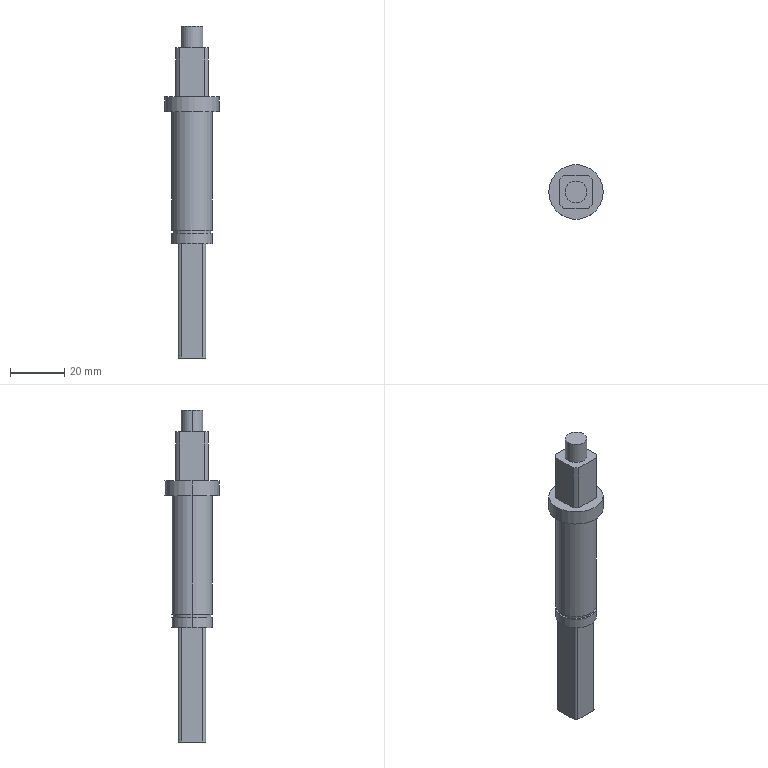Part | STEP file | Drive shaft QY-1-23 | 1 solid | 34 faces | box 20 x 20 x 122 mm | volume 17351 mm3 | cylinder 18 | plane 16 | commonest cylinder face diameters 15 x8 2 x4 8 x2 13.8 x2 20 x2